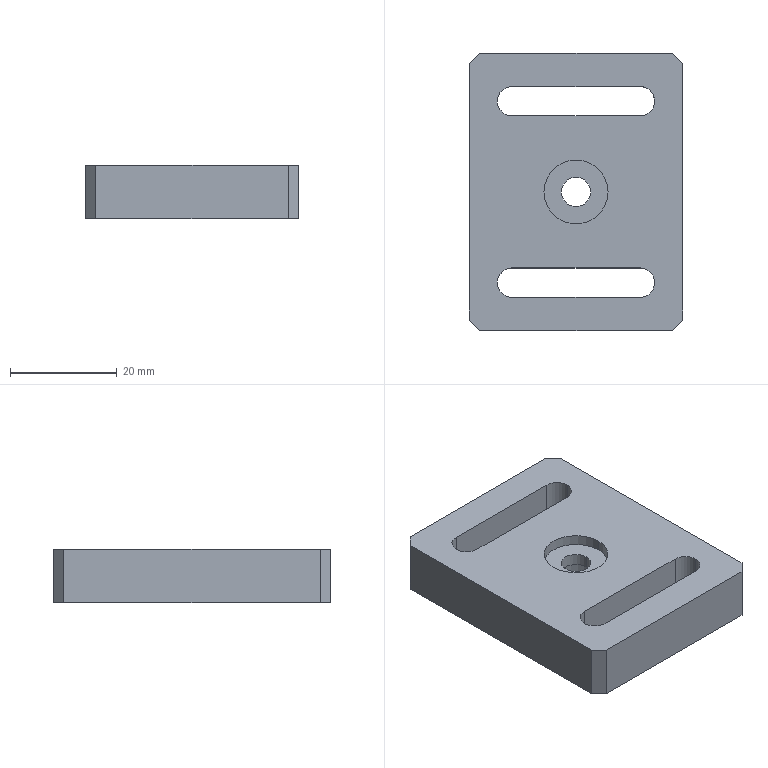Part | STEP file | 11-FG-S00511 | 1 solid | 28 faces | box 40 x 52 x 10 mm | volume 16876 mm3 | plane 16 | cylinder 12 | commonest cylinder face diameters 5.5 x8 10 x2 12 x2
STEP:
#1=CARTESIAN_POINT('',(14.75,-17.,0.));
#2=VERTEX_POINT('',#1);
#3=CARTESIAN_POINT('',(12.,-14.25,0.));
#4=VERTEX_POINT('',#3);
#5=CARTESIAN_POINT('',(12.,-17.,0.));
#6=DIRECTION('',(0.,0.,1.));
#7=DIRECTION('',(1.,0.,0.));
#8=AXIS2_PLACEMENT_3D('',#5,#6,#7);
#9=CIRCLE('',#8,2.75);
#10=EDGE_CURVE('',#2,#4,#9,.T.);
#11=ORIENTED_EDGE('',*,*,#10,.F.);
#12=CARTESIAN_POINT('',(14.75,-17.,10.));
#13=VERTEX_POINT('',#12);
#14=CARTESIAN_POINT('',(14.75,-17.,0.));
#15=DIRECTION('',(0.,0.,1.));
#16=VECTOR('',#15,1000.);
#17=LINE('',#14,#16);
#18=EDGE_CURVE('',#2,#13,#17,.T.);
#19=ORIENTED_EDGE('',*,*,#18,.T.);
#20=CARTESIAN_POINT('',(12.,-14.25,10.));
#21=VERTEX_POINT('',#20);
#22=CARTESIAN_POINT('',(12.,-17.,10.));
#23=DIRECTION('',(0.,0.,1.));
#24=DIRECTION('',(1.,0.,0.));
#25=AXIS2_PLACEMENT_3D('',#22,#23,#24);
#26=CIRCLE('',#25,2.75);
#27=EDGE_CURVE('',#13,#21,#26,.T.);
#28=ORIENTED_EDGE('',*,*,#27,.T.);
#29=CARTESIAN_POINT('',(12.,-14.25,0.));
#30=DIRECTION('',(0.,0.,1.));
#31=VECTOR('',#30,1000.);
#32=LINE('',#29,#31);
#33=EDGE_CURVE('',#4,#21,#32,.T.);
#34=ORIENTED_EDGE('',*,*,#33,.F.);
#35=EDGE_LOOP('',(#11,#19,#28,#34));
#36=FACE_OUTER_BOUND('',#35,.T.);
#37=CARTESIAN_POINT('',(12.,-17.,0.));
#38=DIRECTION('',(0.,0.,1.));
#39=DIRECTION('',(1.,0.,0.));
#40=AXIS2_PLACEMENT_3D('',#37,#38,#39);
#41=CYLINDRICAL_SURFACE('',#40,2.75);
#42=ADVANCED_FACE('',(#36),#41,.F.);
#43=CARTESIAN_POINT('',(14.75,17.,0.));
#44=VERTEX_POINT('',#43);
#45=CARTESIAN_POINT('',(12.,19.75,0.));
#46=VERTEX_POINT('',#45);
#47=CARTESIAN_POINT('',(12.,17.,0.));
#48=DIRECTION('',(0.,0.,1.));
#49=DIRECTION('',(1.,0.,0.));
#50=AXIS2_PLACEMENT_3D('',#47,#48,#49);
#51=CIRCLE('',#50,2.75);
#52=EDGE_CURVE('',#44,#46,#51,.T.);
#53=ORIENTED_EDGE('',*,*,#52,.F.);
#54=CARTESIAN_POINT('',(14.75,17.,10.));
#55=VERTEX_POINT('',#54);
#56=CARTESIAN_POINT('',(14.75,17.,0.));
#57=DIRECTION('',(0.,0.,1.));
#58=VECTOR('',#57,1000.);
#59=LINE('',#56,#58);
#60=EDGE_CURVE('',#44,#55,#59,.T.);
#61=ORIENTED_EDGE('',*,*,#60,.T.);
#62=CARTESIAN_POINT('',(12.,19.75,10.));
#63=VERTEX_POINT('',#62);
#64=CARTESIAN_POINT('',(12.,17.,10.));
#65=DIRECTION('',(0.,0.,1.));
#66=DIRECTION('',(1.,0.,0.));
#67=AXIS2_PLACEMENT_3D('',#64,#65,#66);
#68=CIRCLE('',#67,2.75);
#69=EDGE_CURVE('',#55,#63,#68,.T.);
#70=ORIENTED_EDGE('',*,*,#69,.T.);
#71=CARTESIAN_POINT('',(12.,19.75,0.));
#72=DIRECTION('',(0.,0.,1.));
#73=VECTOR('',#72,1000.);
#74=LINE('',#71,#73);
#75=EDGE_CURVE('',#46,#63,#74,.T.);
#76=ORIENTED_EDGE('',*,*,#75,.F.);
#77=EDGE_LOOP('',(#53,#61,#70,#76));
#78=FACE_OUTER_BOUND('',#77,.T.);
#79=CARTESIAN_POINT('',(12.,17.,0.));
#80=DIRECTION('',(0.,0.,1.));
#81=DIRECTION('',(1.,0.,0.));
#82=AXIS2_PLACEMENT_3D('',#79,#80,#81);
#83=CYLINDRICAL_SURFACE('',#82,2.75);
#84=ADVANCED_FACE('',(#78),#83,.F.);
#85=CARTESIAN_POINT('',(5.,0.,5.7));
#86=VERTEX_POINT('',#85);
#87=CARTESIAN_POINT('',(-5.,0.,5.7));
#88=VERTEX_POINT('',#87);
#89=CARTESIAN_POINT('',(0.,0.,5.7));
#90=DIRECTION('',(0.,0.,-1.));
#91=DIRECTION('',(-1.,0.,0.));
#92=AXIS2_PLACEMENT_3D('',#89,#90,#91);
#93=CIRCLE('',#92,5.);
#94=EDGE_CURVE('',#86,#88,#93,.T.);
#95=ORIENTED_EDGE('',*,*,#94,.F.);
#96=CARTESIAN_POINT('',(5.,0.,0.));
#97=VERTEX_POINT('',#96);
#98=CARTESIAN_POINT('',(5.,0.,0.));
#99=DIRECTION('',(0.,0.,-1.));
#100=VECTOR('',#99,1000.);
#101=LINE('',#98,#100);
#102=EDGE_CURVE('',#86,#97,#101,.T.);
#103=ORIENTED_EDGE('',*,*,#102,.T.);
#104=CARTESIAN_POINT('',(-5.,0.,0.));
#105=VERTEX_POINT('',#104);
#106=CARTESIAN_POINT('',(0.,0.,0.));
#107=DIRECTION('',(0.,0.,-1.));
#108=DIRECTION('',(-1.,0.,0.));
#109=AXIS2_PLACEMENT_3D('',#106,#107,#108);
#110=CIRCLE('',#109,5.);
#111=EDGE_CURVE('',#97,#105,#110,.T.);
#112=ORIENTED_EDGE('',*,*,#111,.T.);
#113=CARTESIAN_POINT('',(-5.,0.,0.));
#114=DIRECTION('',(0.,0.,-1.));
#115=VECTOR('',#114,1000.);
#116=LINE('',#113,#115);
#117=EDGE_CURVE('',#88,#105,#116,.T.);
#118=ORIENTED_EDGE('',*,*,#117,.F.);
#119=EDGE_LOOP('',(#95,#103,#112,#118));
#120=FACE_OUTER_BOUND('',#119,.T.);
#121=CARTESIAN_POINT('',(0.,0.,0.));
#122=DIRECTION('',(0.,0.,-1.));
#123=DIRECTION('',(-1.,0.,0.));
#124=AXIS2_PLACEMENT_3D('',#121,#122,#123);
#125=CYLINDRICAL_SURFACE('',#124,5.);
#126=ADVANCED_FACE('',(#120),#125,.F.);
#127=CARTESIAN_POINT('',(-2.75,0.,8.));
#128=VERTEX_POINT('',#127);
#129=CARTESIAN_POINT('',(2.75,0.,8.));
#130=VERTEX_POINT('',#129);
#131=CARTESIAN_POINT('',(0.,0.,8.));
#132=DIRECTION('',(0.,0.,1.));
#133=DIRECTION('',(1.,0.,0.));
#134=AXIS2_PLACEMENT_3D('',#131,#132,#133);
#135=CIRCLE('',#134,2.75);
#136=EDGE_CURVE('',#128,#130,#135,.T.);
#137=ORIENTED_EDGE('',*,*,#136,.T.);
#138=CARTESIAN_POINT('',(2.75,0.,5.7));
#139=VERTEX_POINT('',#138);
#140=CARTESIAN_POINT('',(2.75,0.,0.));
#141=DIRECTION('',(0.,0.,-1.));
#142=VECTOR('',#141,1000.);
#143=LINE('',#140,#142);
#144=EDGE_CURVE('',#130,#139,#143,.T.);
#145=ORIENTED_EDGE('',*,*,#144,.T.);
#146=CARTESIAN_POINT('',(-2.75,0.,5.7));
#147=VERTEX_POINT('',#146);
#148=CARTESIAN_POINT('',(0.,0.,5.7));
#149=DIRECTION('',(0.,0.,-1.));
#150=DIRECTION('',(-1.,0.,0.));
#151=AXIS2_PLACEMENT_3D('',#148,#149,#150);
#152=CIRCLE('',#151,2.75);
#153=EDGE_CURVE('',#139,#147,#152,.T.);
#154=ORIENTED_EDGE('',*,*,#153,.T.);
#155=CARTESIAN_POINT('',(-2.75,0.,0.));
#156=DIRECTION('',(0.,0.,-1.));
#157=VECTOR('',#156,1000.);
#158=LINE('',#155,#157);
#159=EDGE_CURVE('',#128,#147,#158,.T.);
#160=ORIENTED_EDGE('',*,*,#159,.F.);
#161=EDGE_LOOP('',(#137,#145,#154,#160));
#162=FACE_OUTER_BOUND('',#161,.T.);
#163=CARTESIAN_POINT('',(0.,0.,0.));
#164=DIRECTION('',(0.,0.,-1.));
#165=DIRECTION('',(-1.,0.,0.));
#166=AXIS2_PLACEMENT_3D('',#163,#164,#165);
#167=CYLINDRICAL_SURFACE('',#166,2.75);
#168=ADVANCED_FACE('',(#162),#167,.F.);
#169=CARTESIAN_POINT('',(-6.,0.,8.));
#170=VERTEX_POINT('',#169);
#171=CARTESIAN_POINT('',(6.,0.,8.));
#172=VERTEX_POINT('',#171);
#173=CARTESIAN_POINT('',(0.,0.,8.));
#174=DIRECTION('',(0.,0.,1.));
#175=DIRECTION('',(1.,0.,0.));
#176=AXIS2_PLACEMENT_3D('',#173,#174,#175);
#177=CIRCLE('',#176,6.);
#178=EDGE_CURVE('',#170,#172,#177,.T.);
#179=ORIENTED_EDGE('',*,*,#178,.F.);
#180=CARTESIAN_POINT('',(-6.,0.,10.));
#181=VERTEX_POINT('',#180);
#182=CARTESIAN_POINT('',(-6.,0.,8.));
#183=DIRECTION('',(0.,0.,1.));
#184=VECTOR('',#183,1000.);
#185=LINE('',#182,#184);
#186=EDGE_CURVE('',#170,#181,#185,.T.);
#187=ORIENTED_EDGE('',*,*,#186,.T.);
#188=CARTESIAN_POINT('',(6.,0.,10.));
#189=VERTEX_POINT('',#188);
#190=CARTESIAN_POINT('',(0.,0.,10.));
#191=DIRECTION('',(0.,0.,1.));
#192=DIRECTION('',(1.,0.,0.));
#193=AXIS2_PLACEMENT_3D('',#190,#191,#192);
#194=CIRCLE('',#193,6.);
#195=EDGE_CURVE('',#181,#189,#194,.T.);
#196=ORIENTED_EDGE('',*,*,#195,.T.);
#197=CARTESIAN_POINT('',(6.,0.,8.));
#198=DIRECTION('',(0.,0.,1.));
#199=VECTOR('',#198,1000.);
#200=LINE('',#197,#199);
#201=EDGE_CURVE('',#172,#189,#200,.T.);
#202=ORIENTED_EDGE('',*,*,#201,.F.);
#203=EDGE_LOOP('',(#179,#187,#196,#202));
#204=FACE_OUTER_BOUND('',#203,.T.);
#205=CARTESIAN_POINT('',(0.,0.,8.));
#206=DIRECTION('',(0.,0.,1.));
#207=DIRECTION('',(1.,0.,0.));
#208=AXIS2_PLACEMENT_3D('',#205,#206,#207);
#209=CYLINDRICAL_SURFACE('',#208,6.);
#210=ADVANCED_FACE('',(#204),#209,.F.);
#211=CARTESIAN_POINT('',(20.,-24.,10.));
#212=VERTEX_POINT('',#211);
#213=CARTESIAN_POINT('',(20.,24.,10.));
#214=VERTEX_POINT('',#213);
#215=CARTESIAN_POINT('',(20.,-26.,10.));
#216=DIRECTION('',(0.,1.,0.));
#217=VECTOR('',#216,1000.);
#218=LINE('',#215,#217);
#219=EDGE_CURVE('',#212,#214,#218,.T.);
#220=ORIENTED_EDGE('',*,*,#219,.F.);
#221=CARTESIAN_POINT('',(20.,-24.,0.));
#222=VERTEX_POINT('',#221);
#223=CARTESIAN_POINT('',(20.,-24.,10.));
#224=DIRECTION('',(0.,0.,-1.));
#225=VECTOR('',#224,1000.);
#226=LINE('',#223,#225);
#227=EDGE_CURVE('',#212,#222,#226,.T.);
#228=ORIENTED_EDGE('',*,*,#227,.T.);
#229=CARTESIAN_POINT('',(20.,24.,0.));
#230=VERTEX_POINT('',#229);
#231=CARTESIAN_POINT('',(20.,-26.,0.));
#232=DIRECTION('',(0.,1.,0.));
#233=VECTOR('',#232,1000.);
#234=LINE('',#231,#233);
#235=EDGE_CURVE('',#222,#230,#234,.T.);
#236=ORIENTED_EDGE('',*,*,#235,.T.);
#237=CARTESIAN_POINT('',(20.,24.,10.));
#238=DIRECTION('',(0.,0.,1.));
#239=VECTOR('',#238,1000.);
#240=LINE('',#237,#239);
#241=EDGE_CURVE('',#230,#214,#240,.T.);
#242=ORIENTED_EDGE('',*,*,#241,.T.);
#243=EDGE_LOOP('',(#220,#228,#236,#242));
#244=FACE_OUTER_BOUND('',#243,.T.);
#245=CARTESIAN_POINT('',(20.,-26.,10.));
#246=DIRECTION('',(-1.,0.,0.));
#247=DIRECTION('',(0.,0.,1.));
#248=AXIS2_PLACEMENT_3D('',#245,#246,#247);
#249=PLANE('',#248);
#250=ADVANCED_FACE('',(#244),#249,.F.);
#251=CARTESIAN_POINT('',(18.,26.,10.));
#252=VERTEX_POINT('',#251);
#253=CARTESIAN_POINT('',(-18.,26.,10.));
#254=VERTEX_POINT('',#253);
#255=CARTESIAN_POINT('',(-20.,26.,10.));
#256=DIRECTION('',(-1.,0.,0.));
#257=VECTOR('',#256,1000.);
#258=LINE('',#255,#257);
#259=EDGE_CURVE('',#252,#254,#258,.T.);
#260=ORIENTED_EDGE('',*,*,#259,.F.);
#261=CARTESIAN_POINT('',(18.,26.,0.));
#262=VERTEX_POINT('',#261);
#263=CARTESIAN_POINT('',(18.,26.,10.));
#264=DIRECTION('',(0.,0.,-1.));
#265=VECTOR('',#264,1000.);
#266=LINE('',#263,#265);
#267=EDGE_CURVE('',#252,#262,#266,.T.);
#268=ORIENTED_EDGE('',*,*,#267,.T.);
#269=CARTESIAN_POINT('',(-18.,26.,0.));
#270=VERTEX_POINT('',#269);
#271=CARTESIAN_POINT('',(-20.,26.,0.));
#272=DIRECTION('',(-1.,0.,0.));
#273=VECTOR('',#272,1000.);
#274=LINE('',#271,#273);
#275=EDGE_CURVE('',#262,#270,#274,.T.);
#276=ORIENTED_EDGE('',*,*,#275,.T.);
#277=CARTESIAN_POINT('',(-18.,26.,10.));
#278=DIRECTION('',(0.,0.,1.));
#279=VECTOR('',#278,1000.);
#280=LINE('',#277,#279);
#281=EDGE_CURVE('',#270,#254,#280,.T.);
#282=ORIENTED_EDGE('',*,*,#281,.T.);
#283=EDGE_LOOP('',(#260,#268,#276,#282));
#284=FACE_OUTER_BOUND('',#283,.T.);
#285=CARTESIAN_POINT('',(-20.,26.,10.));
#286=DIRECTION('',(0.,-1.,0.));
#287=DIRECTION('',(0.,0.,-1.));
#288=AXIS2_PLACEMENT_3D('',#285,#286,#287);
#289=PLANE('',#288);
#290=ADVANCED_FACE('',(#284),#289,.F.);
#291=CARTESIAN_POINT('',(-20.,24.,0.));
#292=VERTEX_POINT('',#291);
#293=CARTESIAN_POINT('',(-20.,-24.,0.));
#294=VERTEX_POINT('',#293);
#295=CARTESIAN_POINT('',(-20.,-26.,0.));
#296=DIRECTION('',(0.,-1.,0.));
#297=VECTOR('',#296,1000.);
#298=LINE('',#295,#297);
#299=EDGE_CURVE('',#292,#294,#298,.T.);
#300=ORIENTED_EDGE('',*,*,#299,.T.);
#301=CARTESIAN_POINT('',(-20.,-24.,10.));
#302=VERTEX_POINT('',#301);
#303=CARTESIAN_POINT('',(-20.,-24.,10.));
#304=DIRECTION('',(0.,0.,1.));
#305=VECTOR('',#304,1000.);
#306=LINE('',#303,#305);
#307=EDGE_CURVE('',#294,#302,#306,.T.);
#308=ORIENTED_EDGE('',*,*,#307,.T.);
#309=CARTESIAN_POINT('',(-20.,24.,10.));
#310=VERTEX_POINT('',#309);
#311=CARTESIAN_POINT('',(-20.,-26.,10.));
#312=DIRECTION('',(0.,-1.,0.));
#313=VECTOR('',#312,1000.);
#314=LINE('',#311,#313);
#315=EDGE_CURVE('',#310,#302,#314,.T.);
#316=ORIENTED_EDGE('',*,*,#315,.F.);
#317=CARTESIAN_POINT('',(-20.,24.,10.));
#318=DIRECTION('',(0.,0.,-1.));
#319=VECTOR('',#318,1000.);
#320=LINE('',#317,#319);
#321=EDGE_CURVE('',#310,#292,#320,.T.);
#322=ORIENTED_EDGE('',*,*,#321,.T.);
#323=EDGE_LOOP('',(#300,#308,#316,#322));
#324=FACE_OUTER_BOUND('',#323,.T.);
#325=CARTESIAN_POINT('',(-20.,-26.,10.));
#326=DIRECTION('',(1.,0.,0.));
#327=DIRECTION('',(0.,0.,-1.));
#328=AXIS2_PLACEMENT_3D('',#325,#326,#327);
#329=PLANE('',#328);
#330=ADVANCED_FACE('',(#324),#329,.F.);
#331=CARTESIAN_POINT('',(-18.,-26.,0.));
#332=VERTEX_POINT('',#331);
#333=CARTESIAN_POINT('',(18.,-26.,0.));
#334=VERTEX_POINT('',#333);
#335=CARTESIAN_POINT('',(-20.,-26.,0.));
#336=DIRECTION('',(1.,0.,0.));
#337=VECTOR('',#336,1000.);
#338=LINE('',#335,#337);
#339=EDGE_CURVE('',#332,#334,#338,.T.);
#340=ORIENTED_EDGE('',*,*,#339,.T.);
#341=CARTESIAN_POINT('',(18.,-26.,10.));
#342=VERTEX_POINT('',#341);
#343=CARTESIAN_POINT('',(18.,-26.,10.));
#344=DIRECTION('',(0.,0.,1.));
#345=VECTOR('',#344,1000.);
#346=LINE('',#343,#345);
#347=EDGE_CURVE('',#334,#342,#346,.T.);
#348=ORIENTED_EDGE('',*,*,#347,.T.);
#349=CARTESIAN_POINT('',(-18.,-26.,10.));
#350=VERTEX_POINT('',#349);
#351=CARTESIAN_POINT('',(-20.,-26.,10.));
#352=DIRECTION('',(1.,0.,0.));
#353=VECTOR('',#352,1000.);
#354=LINE('',#351,#353);
#355=EDGE_CURVE('',#350,#342,#354,.T.);
#356=ORIENTED_EDGE('',*,*,#355,.F.);
#357=CARTESIAN_POINT('',(-18.,-26.,10.));
#358=DIRECTION('',(0.,0.,-1.));
#359=VECTOR('',#358,1000.);
#360=LINE('',#357,#359);
#361=EDGE_CURVE('',#350,#332,#360,.T.);
#362=ORIENTED_EDGE('',*,*,#361,.T.);
#363=EDGE_LOOP('',(#340,#348,#356,#362));
#364=FACE_OUTER_BOUND('',#363,.T.);
#365=CARTESIAN_POINT('',(-20.,-26.,10.));
#366=DIRECTION('',(0.,1.,0.));
#367=DIRECTION('',(0.,0.,1.));
#368=AXIS2_PLACEMENT_3D('',#365,#366,#367);
#369=PLANE('',#368);
#370=ADVANCED_FACE('',(#364),#369,.F.);
#371=CARTESIAN_POINT('',(-12.,-14.25,10.));
#372=VERTEX_POINT('',#371);
#373=CARTESIAN_POINT('',(12.,-14.25,10.));
#374=DIRECTION('',(-1.,0.,0.));
#375=VECTOR('',#374,1000.);
#376=LINE('',#373,#375);
#377=EDGE_CURVE('',#21,#372,#376,.T.);
#378=ORIENTED_EDGE('',*,*,#377,.F.);
#379=ORIENTED_EDGE('',*,*,#27,.F.);
#380=CARTESIAN_POINT('',(12.,-19.75,10.));
#381=VERTEX_POINT('',#380);
#382=CARTESIAN_POINT('',(12.,-17.,10.));
#383=DIRECTION('',(0.,0.,1.));
#384=DIRECTION('',(1.,0.,0.));
#385=AXIS2_PLACEMENT_3D('',#382,#383,#384);
#386=CIRCLE('',#385,2.75);
#387=EDGE_CURVE('',#381,#13,#386,.T.);
#388=ORIENTED_EDGE('',*,*,#387,.F.);
#389=CARTESIAN_POINT('',(-12.,-19.75,10.));
#390=VERTEX_POINT('',#389);
#391=CARTESIAN_POINT('',(12.,-19.75,10.));
#392=DIRECTION('',(1.,0.,0.));
#393=VECTOR('',#392,1000.);
#394=LINE('',#391,#393);
#395=EDGE_CURVE('',#390,#381,#394,.T.);
#396=ORIENTED_EDGE('',*,*,#395,.F.);
#397=CARTESIAN_POINT('',(-12.,-17.,10.));
#398=DIRECTION('',(0.,0.,1.));
#399=DIRECTION('',(1.,0.,0.));
#400=AXIS2_PLACEMENT_3D('',#397,#398,#399);
#401=CIRCLE('',#400,2.75);
#402=EDGE_CURVE('',#372,#390,#401,.T.);
#403=ORIENTED_EDGE('',*,*,#402,.F.);
#404=EDGE_LOOP('',(#378,#379,#388,#396,#403));
#405=FACE_BOUND('',#404,.T.);
#406=CARTESIAN_POINT('',(-12.,19.75,10.));
#407=VERTEX_POINT('',#406);
#408=CARTESIAN_POINT('',(12.,19.75,10.));
#409=DIRECTION('',(-1.,0.,0.));
#410=VECTOR('',#409,1000.);
#411=LINE('',#408,#410);
#412=EDGE_CURVE('',#63,#407,#411,.T.);
#413=ORIENTED_EDGE('',*,*,#412,.F.);
#414=ORIENTED_EDGE('',*,*,#69,.F.);
#415=CARTESIAN_POINT('',(12.,14.25,10.));
#416=VERTEX_POINT('',#415);
#417=CARTESIAN_POINT('',(12.,17.,10.));
#418=DIRECTION('',(0.,0.,1.));
#419=DIRECTION('',(1.,0.,0.));
#420=AXIS2_PLACEMENT_3D('',#417,#418,#419);
#421=CIRCLE('',#420,2.75);
#422=EDGE_CURVE('',#416,#55,#421,.T.);
#423=ORIENTED_EDGE('',*,*,#422,.F.);
#424=CARTESIAN_POINT('',(-12.,14.25,10.));
#425=VERTEX_POINT('',#424);
#426=CARTESIAN_POINT('',(12.,14.25,10.));
#427=DIRECTION('',(1.,0.,0.));
#428=VECTOR('',#427,1000.);
#429=LINE('',#426,#428);
#430=EDGE_CURVE('',#425,#416,#429,.T.);
#431=ORIENTED_EDGE('',*,*,#430,.F.);
#432=CARTESIAN_POINT('',(-12.,17.,10.));
#433=DIRECTION('',(0.,0.,1.));
#434=DIRECTION('',(1.,0.,0.));
#435=AXIS2_PLACEMENT_3D('',#432,#433,#434);
#436=CIRCLE('',#435,2.75);
#437=EDGE_CURVE('',#407,#425,#436,.T.);
#438=ORIENTED_EDGE('',*,*,#437,.F.);
#439=EDGE_LOOP('',(#413,#414,#423,#431,#438));
#440=FACE_BOUND('',#439,.T.);
#441=CARTESIAN_POINT('',(0.,0.,10.));
#442=DIRECTION('',(0.,0.,1.));
#443=DIRECTION('',(1.,0.,0.));
#444=AXIS2_PLACEMENT_3D('',#441,#442,#443);
#445=CIRCLE('',#444,6.);
#446=EDGE_CURVE('',#189,#181,#445,.T.);
#447=ORIENTED_EDGE('',*,*,#446,.F.);
#448=ORIENTED_EDGE('',*,*,#195,.F.);
#449=EDGE_LOOP('',(#447,#448));
#450=FACE_BOUND('',#449,.T.);
#451=ORIENTED_EDGE('',*,*,#355,.T.);
#452=CARTESIAN_POINT('',(20.,-24.,10.));
#453=DIRECTION('',(0.7071,0.7071,0.));
#454=VECTOR('',#453,1000.);
#455=LINE('',#452,#454);
#456=EDGE_CURVE('',#342,#212,#455,.T.);
#457=ORIENTED_EDGE('',*,*,#456,.T.);
#458=ORIENTED_EDGE('',*,*,#219,.T.);
#459=CARTESIAN_POINT('',(18.,26.,10.));
#460=DIRECTION('',(-0.7071,0.7071,0.));
#461=VECTOR('',#460,1000.);
#462=LINE('',#459,#461);
#463=EDGE_CURVE('',#214,#252,#462,.T.);
#464=ORIENTED_EDGE('',*,*,#463,.T.);
#465=ORIENTED_EDGE('',*,*,#259,.T.);
#466=CARTESIAN_POINT('',(-20.,24.,10.));
#467=DIRECTION('',(-0.7071,-0.7071,0.));
#468=VECTOR('',#467,1000.);
#469=LINE('',#466,#468);
#470=EDGE_CURVE('',#254,#310,#469,.T.);
#471=ORIENTED_EDGE('',*,*,#470,.T.);
#472=ORIENTED_EDGE('',*,*,#315,.T.);
#473=CARTESIAN_POINT('',(-18.,-26.,10.));
#474=DIRECTION('',(0.7071,-0.7071,0.));
#475=VECTOR('',#474,1000.);
#476=LINE('',#473,#475);
#477=EDGE_CURVE('',#302,#350,#476,.T.);
#478=ORIENTED_EDGE('',*,*,#477,.T.);
#479=EDGE_LOOP('',(#451,#457,#458,#464,#465,#471,#472,#478));
#480=FACE_OUTER_BOUND('',#479,.T.);
#481=CARTESIAN_POINT('',(0.,0.,10.));
#482=DIRECTION('',(0.,0.,-1.));
#483=DIRECTION('',(-1.,0.,0.));
#484=AXIS2_PLACEMENT_3D('',#481,#482,#483);
#485=PLANE('',#484);
#486=ADVANCED_FACE('',(#405,#440,#450,#480),#485,.F.);
#487=CARTESIAN_POINT('',(12.,-19.75,0.));
#488=VERTEX_POINT('',#487);
#489=CARTESIAN_POINT('',(12.,-17.,0.));
#490=DIRECTION('',(0.,0.,1.));
#491=DIRECTION('',(1.,0.,0.));
#492=AXIS2_PLACEMENT_3D('',#489,#490,#491);
#493=CIRCLE('',#492,2.75);
#494=EDGE_CURVE('',#488,#2,#493,.T.);
#495=ORIENTED_EDGE('',*,*,#494,.T.);
#496=ORIENTED_EDGE('',*,*,#10,.T.);
#497=CARTESIAN_POINT('',(-12.,-14.25,0.));
#498=VERTEX_POINT('',#497);
#499=CARTESIAN_POINT('',(12.,-14.25,0.));
#500=DIRECTION('',(-1.,0.,0.));
#501=VECTOR('',#500,1000.);
#502=LINE('',#499,#501);
#503=EDGE_CURVE('',#4,#498,#502,.T.);
#504=ORIENTED_EDGE('',*,*,#503,.T.);
#505=CARTESIAN_POINT('',(-12.,-19.75,0.));
#506=VERTEX_POINT('',#505);
#507=CARTESIAN_POINT('',(-12.,-17.,0.));
#508=DIRECTION('',(0.,0.,1.));
#509=DIRECTION('',(1.,0.,0.));
#510=AXIS2_PLACEMENT_3D('',#507,#508,#509);
#511=CIRCLE('',#510,2.75);
#512=EDGE_CURVE('',#498,#506,#511,.T.);
#513=ORIENTED_EDGE('',*,*,#512,.T.);
#514=CARTESIAN_POINT('',(12.,-19.75,0.));
#515=DIRECTION('',(1.,0.,0.));
#516=VECTOR('',#515,1000.);
#517=LINE('',#514,#516);
#518=EDGE_CURVE('',#506,#488,#517,.T.);
#519=ORIENTED_EDGE('',*,*,#518,.T.);
#520=EDGE_LOOP('',(#495,#496,#504,#513,#519));
#521=FACE_BOUND('',#520,.T.);
#522=CARTESIAN_POINT('',(12.,14.25,0.));
#523=VERTEX_POINT('',#522);
#524=CARTESIAN_POINT('',(12.,17.,0.));
#525=DIRECTION('',(0.,0.,1.));
#526=DIRECTION('',(1.,0.,0.));
#527=AXIS2_PLACEMENT_3D('',#524,#525,#526);
#528=CIRCLE('',#527,2.75);
#529=EDGE_CURVE('',#523,#44,#528,.T.);
#530=ORIENTED_EDGE('',*,*,#529,.T.);
#531=ORIENTED_EDGE('',*,*,#52,.T.);
#532=CARTESIAN_POINT('',(-12.,19.75,0.));
#533=VERTEX_POINT('',#532);
#534=CARTESIAN_POINT('',(12.,19.75,0.));
#535=DIRECTION('',(-1.,0.,0.));
#536=VECTOR('',#535,1000.);
#537=LINE('',#534,#536);
#538=EDGE_CURVE('',#46,#533,#537,.T.);
#539=ORIENTED_EDGE('',*,*,#538,.T.);
#540=CARTESIAN_POINT('',(-12.,14.25,0.));
#541=VERTEX_POINT('',#540);
#542=CARTESIAN_POINT('',(-12.,17.,0.));
#543=DIRECTION('',(0.,0.,1.));
#544=DIRECTION('',(1.,0.,0.));
#545=AXIS2_PLACEMENT_3D('',#542,#543,#544);
#546=CIRCLE('',#545,2.75);
#547=EDGE_CURVE('',#533,#541,#546,.T.);
#548=ORIENTED_EDGE('',*,*,#547,.T.);
#549=CARTESIAN_POINT('',(12.,14.25,0.));
#550=DIRECTION('',(1.,0.,0.));
#551=VECTOR('',#550,1000.);
#552=LINE('',#549,#551);
#553=EDGE_CURVE('',#541,#523,#552,.T.);
#554=ORIENTED_EDGE('',*,*,#553,.T.);
#555=EDGE_LOOP('',(#530,#531,#539,#548,#554));
#556=FACE_BOUND('',#555,.T.);
#557=CARTESIAN_POINT('',(0.,0.,0.));
#558=DIRECTION('',(0.,0.,-1.));
#559=DIRECTION('',(-1.,0.,0.));
#560=AXIS2_PLACEMENT_3D('',#557,#558,#559);
#561=CIRCLE('',#560,5.);
#562=EDGE_CURVE('',#105,#97,#561,.T.);
#563=ORIENTED_EDGE('',*,*,#562,.F.);
#564=ORIENTED_EDGE('',*,*,#111,.F.);
#565=EDGE_LOOP('',(#563,#564));
#566=FACE_BOUND('',#565,.T.);
#567=ORIENTED_EDGE('',*,*,#235,.F.);
#568=CARTESIAN_POINT('',(22.,-22.,0.));
#569=DIRECTION('',(-0.7071,-0.7071,0.));
#570=VECTOR('',#569,1000.);
#571=LINE('',#568,#570);
#572=EDGE_CURVE('',#222,#334,#571,.T.);
#573=ORIENTED_EDGE('',*,*,#572,.T.);
#574=ORIENTED_EDGE('',*,*,#339,.F.);
#575=CARTESIAN_POINT('',(-22.,-22.,0.));
#576=DIRECTION('',(-0.7071,0.7071,0.));
#577=VECTOR('',#576,1000.);
#578=LINE('',#575,#577);
#579=EDGE_CURVE('',#332,#294,#578,.T.);
#580=ORIENTED_EDGE('',*,*,#579,.T.);
#581=ORIENTED_EDGE('',*,*,#299,.F.);
#582=CARTESIAN_POINT('',(-22.,22.,0.));
#583=DIRECTION('',(0.7071,0.7071,0.));
#584=VECTOR('',#583,1000.);
#585=LINE('',#582,#584);
#586=EDGE_CURVE('',#292,#270,#585,.T.);
#587=ORIENTED_EDGE('',*,*,#586,.T.);
#588=ORIENTED_EDGE('',*,*,#275,.F.);
#589=CARTESIAN_POINT('',(22.,22.,0.));
#590=DIRECTION('',(0.7071,-0.7071,0.));
#591=VECTOR('',#590,1000.);
#592=LINE('',#589,#591);
#593=EDGE_CURVE('',#262,#230,#592,.T.);
#594=ORIENTED_EDGE('',*,*,#593,.T.);
#595=EDGE_LOOP('',(#567,#573,#574,#580,#581,#587,#588,#594));
#596=FACE_OUTER_BOUND('',#595,.T.);
#597=CARTESIAN_POINT('',(0.,0.,0.));
#598=DIRECTION('',(0.,0.,-1.));
#599=DIRECTION('',(-1.,0.,0.));
#600=AXIS2_PLACEMENT_3D('',#597,#598,#599);
#601=PLANE('',#600);
#602=ADVANCED_FACE('',(#521,#556,#566,#596),#601,.T.);
#603=ORIENTED_EDGE('',*,*,#456,.F.);
#604=ORIENTED_EDGE('',*,*,#347,.F.);
#605=ORIENTED_EDGE('',*,*,#572,.F.);
#606=ORIENTED_EDGE('',*,*,#227,.F.);
#607=EDGE_LOOP('',(#603,#604,#605,#606));
#608=FACE_OUTER_BOUND('',#607,.T.);
#609=CARTESIAN_POINT('',(20.,-24.,10.));
#610=DIRECTION('',(-0.7071,0.7071,0.));
#611=DIRECTION('',(0.,0.,-1.));
#612=AXIS2_PLACEMENT_3D('',#609,#610,#611);
#613=PLANE('',#612);
#614=ADVANCED_FACE('',(#608),#613,.F.);
#615=ORIENTED_EDGE('',*,*,#463,.F.);
#616=ORIENTED_EDGE('',*,*,#241,.F.);
#617=ORIENTED_EDGE('',*,*,#593,.F.);
#618=ORIENTED_EDGE('',*,*,#267,.F.);
#619=EDGE_LOOP('',(#615,#616,#617,#618));
#620=FACE_OUTER_BOUND('',#619,.T.);
#621=CARTESIAN_POINT('',(18.,26.,10.));
#622=DIRECTION('',(-0.7071,-0.7071,0.));
#623=DIRECTION('',(0.,0.,-1.));
#624=AXIS2_PLACEMENT_3D('',#621,#622,#623);
#625=PLANE('',#624);
#626=ADVANCED_FACE('',(#620),#625,.F.);
#627=ORIENTED_EDGE('',*,*,#477,.F.);
#628=ORIENTED_EDGE('',*,*,#307,.F.);
#629=ORIENTED_EDGE('',*,*,#579,.F.);
#630=ORIENTED_EDGE('',*,*,#361,.F.);
#631=EDGE_LOOP('',(#627,#628,#629,#630));
#632=FACE_OUTER_BOUND('',#631,.T.);
#633=CARTESIAN_POINT('',(-18.,-26.,10.));
#634=DIRECTION('',(0.7071,0.7071,0.));
#635=DIRECTION('',(0.,0.,-1.));
#636=AXIS2_PLACEMENT_3D('',#633,#634,#635);
#637=PLANE('',#636);
#638=ADVANCED_FACE('',(#632),#637,.F.);
#639=ORIENTED_EDGE('',*,*,#470,.F.);
#640=ORIENTED_EDGE('',*,*,#281,.F.);
#641=ORIENTED_EDGE('',*,*,#586,.F.);
#642=ORIENTED_EDGE('',*,*,#321,.F.);
#643=EDGE_LOOP('',(#639,#640,#641,#642));
#644=FACE_OUTER_BOUND('',#643,.T.);
#645=CARTESIAN_POINT('',(-20.,24.,10.));
#646=DIRECTION('',(0.7071,-0.7071,0.));
#647=DIRECTION('',(0.,0.,-1.));
#648=AXIS2_PLACEMENT_3D('',#645,#646,#647);
#649=PLANE('',#648);
#650=ADVANCED_FACE('',(#644),#649,.F.);
#651=ORIENTED_EDGE('',*,*,#186,.F.);
#652=CARTESIAN_POINT('',(0.,0.,8.));
#653=DIRECTION('',(0.,0.,1.));
#654=DIRECTION('',(1.,0.,0.));
#655=AXIS2_PLACEMENT_3D('',#652,#653,#654);
#656=CIRCLE('',#655,6.);
#657=EDGE_CURVE('',#172,#170,#656,.T.);
#658=ORIENTED_EDGE('',*,*,#657,.F.);
#659=ORIENTED_EDGE('',*,*,#201,.T.);
#660=ORIENTED_EDGE('',*,*,#446,.T.);
#661=EDGE_LOOP('',(#651,#658,#659,#660));
#662=FACE_OUTER_BOUND('',#661,.T.);
#663=CARTESIAN_POINT('',(0.,0.,8.));
#664=DIRECTION('',(0.,0.,1.));
#665=DIRECTION('',(1.,0.,0.));
#666=AXIS2_PLACEMENT_3D('',#663,#664,#665);
#667=CYLINDRICAL_SURFACE('',#666,6.);
#668=ADVANCED_FACE('',(#662),#667,.F.);
#669=ORIENTED_EDGE('',*,*,#136,.F.);
#670=CARTESIAN_POINT('',(0.,0.,8.));
#671=DIRECTION('',(0.,0.,1.));
#672=DIRECTION('',(1.,0.,0.));
#673=AXIS2_PLACEMENT_3D('',#670,#671,#672);
#674=CIRCLE('',#673,2.75);
#675=EDGE_CURVE('',#130,#128,#674,.T.);
#676=ORIENTED_EDGE('',*,*,#675,.F.);
#677=EDGE_LOOP('',(#669,#676));
#678=FACE_BOUND('',#677,.T.);
#679=ORIENTED_EDGE('',*,*,#657,.T.);
#680=ORIENTED_EDGE('',*,*,#178,.T.);
#681=EDGE_LOOP('',(#679,#680));
#682=FACE_OUTER_BOUND('',#681,.T.);
#683=CARTESIAN_POINT('',(0.,0.,8.));
#684=DIRECTION('',(0.,0.,1.));
#685=DIRECTION('',(1.,0.,0.));
#686=AXIS2_PLACEMENT_3D('',#683,#684,#685);
#687=PLANE('',#686);
#688=ADVANCED_FACE('',(#678,#682),#687,.T.);
#689=ORIENTED_EDGE('',*,*,#144,.F.);
#690=ORIENTED_EDGE('',*,*,#675,.T.);
#691=ORIENTED_EDGE('',*,*,#159,.T.);
#692=CARTESIAN_POINT('',(0.,0.,5.7));
#693=DIRECTION('',(0.,0.,-1.));
#694=DIRECTION('',(-1.,0.,0.));
#695=AXIS2_PLACEMENT_3D('',#692,#693,#694);
#696=CIRCLE('',#695,2.75);
#697=EDGE_CURVE('',#147,#139,#696,.T.);
#698=ORIENTED_EDGE('',*,*,#697,.T.);
#699=EDGE_LOOP('',(#689,#690,#691,#698));
#700=FACE_OUTER_BOUND('',#699,.T.);
#701=CARTESIAN_POINT('',(0.,0.,0.));
#702=DIRECTION('',(0.,0.,-1.));
#703=DIRECTION('',(-1.,0.,0.));
#704=AXIS2_PLACEMENT_3D('',#701,#702,#703);
#705=CYLINDRICAL_SURFACE('',#704,2.75);
#706=ADVANCED_FACE('',(#700),#705,.F.);
#707=ORIENTED_EDGE('',*,*,#697,.F.);
#708=ORIENTED_EDGE('',*,*,#153,.F.);
#709=EDGE_LOOP('',(#707,#708));
#710=FACE_BOUND('',#709,.T.);
#711=CARTESIAN_POINT('',(0.,0.,5.7));
#712=DIRECTION('',(0.,0.,-1.));
#713=DIRECTION('',(-1.,0.,0.));
#714=AXIS2_PLACEMENT_3D('',#711,#712,#713);
#715=CIRCLE('',#714,5.);
#716=EDGE_CURVE('',#88,#86,#715,.T.);
#717=ORIENTED_EDGE('',*,*,#716,.T.);
#718=ORIENTED_EDGE('',*,*,#94,.T.);
#719=EDGE_LOOP('',(#717,#718));
#720=FACE_OUTER_BOUND('',#719,.T.);
#721=CARTESIAN_POINT('',(2.75,0.,5.7));
#722=DIRECTION('',(0.,0.,1.));
#723=DIRECTION('',(1.,0.,0.));
#724=AXIS2_PLACEMENT_3D('',#721,#722,#723);
#725=PLANE('',#724);
#726=ADVANCED_FACE('',(#710,#720),#725,.F.);
#727=ORIENTED_EDGE('',*,*,#102,.F.);
#728=ORIENTED_EDGE('',*,*,#716,.F.);
#729=ORIENTED_EDGE('',*,*,#117,.T.);
#730=ORIENTED_EDGE('',*,*,#562,.T.);
#731=EDGE_LOOP('',(#727,#728,#729,#730));
#732=FACE_OUTER_BOUND('',#731,.T.);
#733=CARTESIAN_POINT('',(0.,0.,0.));
#734=DIRECTION('',(0.,0.,-1.));
#735=DIRECTION('',(-1.,0.,0.));
#736=AXIS2_PLACEMENT_3D('',#733,#734,#735);
#737=CYLINDRICAL_SURFACE('',#736,5.);
#738=ADVANCED_FACE('',(#732),#737,.F.);
#739=ORIENTED_EDGE('',*,*,#60,.F.);
#740=ORIENTED_EDGE('',*,*,#529,.F.);
#741=CARTESIAN_POINT('',(12.,14.25,0.));
#742=DIRECTION('',(0.,0.,1.));
#743=VECTOR('',#742,1000.);
#744=LINE('',#741,#743);
#745=EDGE_CURVE('',#523,#416,#744,.T.);
#746=ORIENTED_EDGE('',*,*,#745,.T.);
#747=ORIENTED_EDGE('',*,*,#422,.T.);
#748=EDGE_LOOP('',(#739,#740,#746,#747));
#749=FACE_OUTER_BOUND('',#748,.T.);
#750=CARTESIAN_POINT('',(12.,17.,0.));
#751=DIRECTION('',(0.,0.,1.));
#752=DIRECTION('',(1.,0.,0.));
#753=AXIS2_PLACEMENT_3D('',#750,#751,#752);
#754=CYLINDRICAL_SURFACE('',#753,2.75);
#755=ADVANCED_FACE('',(#749),#754,.F.);
#756=ORIENTED_EDGE('',*,*,#430,.T.);
#757=ORIENTED_EDGE('',*,*,#745,.F.);
#758=ORIENTED_EDGE('',*,*,#553,.F.);
#759=CARTESIAN_POINT('',(-12.,14.25,0.));
#760=DIRECTION('',(0.,0.,1.));
#761=VECTOR('',#760,1000.);
#762=LINE('',#759,#761);
#763=EDGE_CURVE('',#541,#425,#762,.T.);
#764=ORIENTED_EDGE('',*,*,#763,.T.);
#765=EDGE_LOOP('',(#756,#757,#758,#764));
#766=FACE_OUTER_BOUND('',#765,.T.);
#767=CARTESIAN_POINT('',(12.,14.25,0.));
#768=DIRECTION('',(0.,-1.,0.));
#769=DIRECTION('',(0.,0.,-1.));
#770=AXIS2_PLACEMENT_3D('',#767,#768,#769);
#771=PLANE('',#770);
#772=ADVANCED_FACE('',(#766),#771,.F.);
#773=ORIENTED_EDGE('',*,*,#437,.T.);
#774=ORIENTED_EDGE('',*,*,#763,.F.);
#775=ORIENTED_EDGE('',*,*,#547,.F.);
#776=CARTESIAN_POINT('',(-12.,19.75,0.));
#777=DIRECTION('',(0.,0.,1.));
#778=VECTOR('',#777,1000.);
#779=LINE('',#776,#778);
#780=EDGE_CURVE('',#533,#407,#779,.T.);
#781=ORIENTED_EDGE('',*,*,#780,.T.);
#782=EDGE_LOOP('',(#773,#774,#775,#781));
#783=FACE_OUTER_BOUND('',#782,.T.);
#784=CARTESIAN_POINT('',(-12.,17.,0.));
#785=DIRECTION('',(0.,0.,1.));
#786=DIRECTION('',(1.,0.,0.));
#787=AXIS2_PLACEMENT_3D('',#784,#785,#786);
#788=CYLINDRICAL_SURFACE('',#787,2.75);
#789=ADVANCED_FACE('',(#783),#788,.F.);
#790=ORIENTED_EDGE('',*,*,#412,.T.);
#791=ORIENTED_EDGE('',*,*,#780,.F.);
#792=ORIENTED_EDGE('',*,*,#538,.F.);
#793=ORIENTED_EDGE('',*,*,#75,.T.);
#794=EDGE_LOOP('',(#790,#791,#792,#793));
#795=FACE_OUTER_BOUND('',#794,.T.);
#796=CARTESIAN_POINT('',(12.,19.75,0.));
#797=DIRECTION('',(0.,1.,0.));
#798=DIRECTION('',(0.,0.,1.));
#799=AXIS2_PLACEMENT_3D('',#796,#797,#798);
#800=PLANE('',#799);
#801=ADVANCED_FACE('',(#795),#800,.F.);
#802=ORIENTED_EDGE('',*,*,#18,.F.);
#803=ORIENTED_EDGE('',*,*,#494,.F.);
#804=CARTESIAN_POINT('',(12.,-19.75,0.));
#805=DIRECTION('',(0.,0.,1.));
#806=VECTOR('',#805,1000.);
#807=LINE('',#804,#806);
#808=EDGE_CURVE('',#488,#381,#807,.T.);
#809=ORIENTED_EDGE('',*,*,#808,.T.);
#810=ORIENTED_EDGE('',*,*,#387,.T.);
#811=EDGE_LOOP('',(#802,#803,#809,#810));
#812=FACE_OUTER_BOUND('',#811,.T.);
#813=CARTESIAN_POINT('',(12.,-17.,0.));
#814=DIRECTION('',(0.,0.,1.));
#815=DIRECTION('',(1.,0.,0.));
#816=AXIS2_PLACEMENT_3D('',#813,#814,#815);
#817=CYLINDRICAL_SURFACE('',#816,2.75);
#818=ADVANCED_FACE('',(#812),#817,.F.);
#819=ORIENTED_EDGE('',*,*,#395,.T.);
#820=ORIENTED_EDGE('',*,*,#808,.F.);
#821=ORIENTED_EDGE('',*,*,#518,.F.);
#822=CARTESIAN_POINT('',(-12.,-19.75,0.));
#823=DIRECTION('',(0.,0.,1.));
#824=VECTOR('',#823,1000.);
#825=LINE('',#822,#824);
#826=EDGE_CURVE('',#506,#390,#825,.T.);
#827=ORIENTED_EDGE('',*,*,#826,.T.);
#828=EDGE_LOOP('',(#819,#820,#821,#827));
#829=FACE_OUTER_BOUND('',#828,.T.);
#830=CARTESIAN_POINT('',(12.,-19.75,0.));
#831=DIRECTION('',(0.,-1.,0.));
#832=DIRECTION('',(0.,0.,-1.));
#833=AXIS2_PLACEMENT_3D('',#830,#831,#832);
#834=PLANE('',#833);
#835=ADVANCED_FACE('',(#829),#834,.F.);
#836=ORIENTED_EDGE('',*,*,#402,.T.);
#837=ORIENTED_EDGE('',*,*,#826,.F.);
#838=ORIENTED_EDGE('',*,*,#512,.F.);
#839=CARTESIAN_POINT('',(-12.,-14.25,0.));
#840=DIRECTION('',(0.,0.,1.));
#841=VECTOR('',#840,1000.);
#842=LINE('',#839,#841);
#843=EDGE_CURVE('',#498,#372,#842,.T.);
#844=ORIENTED_EDGE('',*,*,#843,.T.);
#845=EDGE_LOOP('',(#836,#837,#838,#844));
#846=FACE_OUTER_BOUND('',#845,.T.);
#847=CARTESIAN_POINT('',(-12.,-17.,0.));
#848=DIRECTION('',(0.,0.,1.));
#849=DIRECTION('',(1.,0.,0.));
#850=AXIS2_PLACEMENT_3D('',#847,#848,#849);
#851=CYLINDRICAL_SURFACE('',#850,2.75);
#852=ADVANCED_FACE('',(#846),#851,.F.);
#853=ORIENTED_EDGE('',*,*,#377,.T.);
#854=ORIENTED_EDGE('',*,*,#843,.F.);
#855=ORIENTED_EDGE('',*,*,#503,.F.);
#856=ORIENTED_EDGE('',*,*,#33,.T.);
#857=EDGE_LOOP('',(#853,#854,#855,#856));
#858=FACE_OUTER_BOUND('',#857,.T.);
#859=CARTESIAN_POINT('',(12.,-14.25,0.));
#860=DIRECTION('',(0.,1.,0.));
#861=DIRECTION('',(0.,0.,1.));
#862=AXIS2_PLACEMENT_3D('',#859,#860,#861);
#863=PLANE('',#862);
#864=ADVANCED_FACE('',(#858),#863,.F.);
#865=CLOSED_SHELL('',(#42,#84,#126,#168,#210,#250,#290,#330,#370,#486,#602,#614,#626,#638,#650,#668,#688,#706,#726,#738,#755,#772,#789,#801,#818,#835,#852,#864));
#866=MANIFOLD_SOLID_BREP('',#865);
#867=CARTESIAN_POINT('',(0.,0.,0.));
#868=DIRECTION('',(0.,0.,1.));
#869=DIRECTION('',(1.,0.,0.));
#870=AXIS2_PLACEMENT_3D('',#867,#868,#869);
#871=(LENGTH_UNIT()NAMED_UNIT(*)SI_UNIT(.MILLI.,.METRE.));
#872=UNCERTAINTY_MEASURE_WITH_UNIT(LENGTH_MEASURE(0.00001),#871,'','');
#873=(NAMED_UNIT(*)PLANE_ANGLE_UNIT()SI_UNIT($,.RADIAN.));
#874=(NAMED_UNIT(*)SI_UNIT($,.STERADIAN.)SOLID_ANGLE_UNIT());
#875=(GEOMETRIC_REPRESENTATION_CONTEXT(3)GLOBAL_UNCERTAINTY_ASSIGNED_CONTEXT((#872))GLOBAL_UNIT_ASSIGNED_CONTEXT((#871,#873,#874))REPRESENTATION_CONTEXT('',''));
#876=ADVANCED_BREP_SHAPE_REPRESENTATION('',(#866,#870),#875);